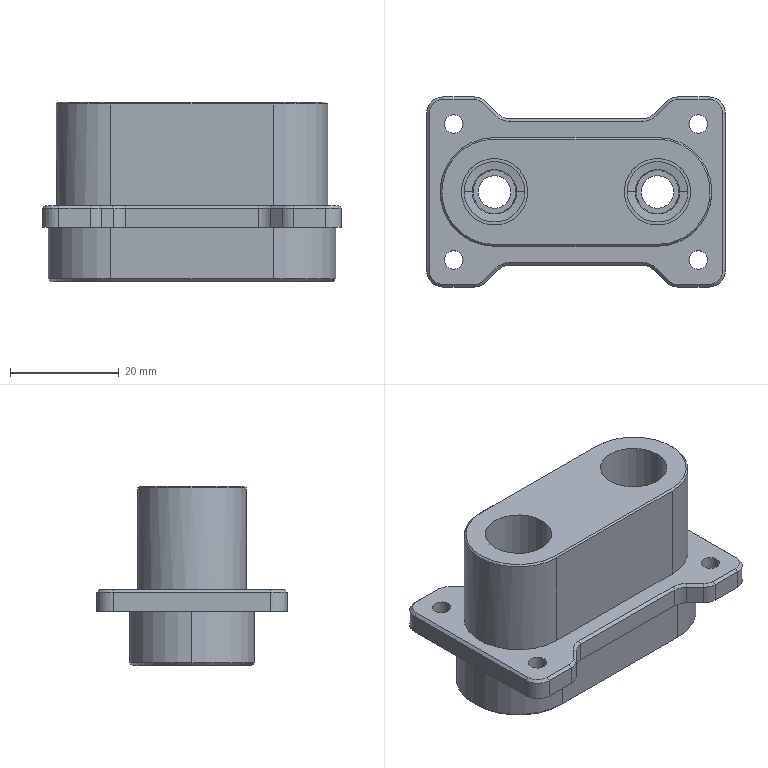NC program | NX | posted with a generic post | part box 55 x 35 x 33 mm
Lines 1 to 866 of 2805:
N10 G17 G21 G94 G90
(ADAPTIVE_MILLING_COPY , TOOL : D6开粗)
N12 T02 M6
N14 G54
N16 G17 G0 G90 X0.026 Y-37.084 S5500 M3
N18 G43 Z30. H2
N20 Z-5.425
N22 G94 G1 X0.007 Y-36.935 Z-6.362 F2500.
N24 X-0.012 Y-36.787 Z-6.733
N26 X-0.03 Y-36.638 Z-7.005
N28 X-0.049 Y-36.489 Z-7.225
N30 X-0.067 Y-36.34 Z-7.409
N32 X-0.086 Y-36.191 Z-7.567
N34 X-0.104 Y-36.042 Z-7.705
N36 X-0.123 Y-35.893 Z-7.825
N38 X-0.142 Y-35.745 Z-7.93
N40 X-0.16 Y-35.596 Z-8.023
N42 X-0.179 Y-35.447 Z-8.104
N44 X-0.197 Y-35.298 Z-8.175
N46 X-0.216 Y-35.149 Z-8.235
N48 X-0.235 Y-35. Z-8.287
N50 X-0.253 Y-34.852 Z-8.33
N52 X-0.272 Y-34.703 Z-8.364
N54 X-0.29 Y-34.554 Z-8.391
N56 X-0.309 Y-34.405 Z-8.41
N58 X-0.327 Y-34.256 Z-8.421
N60 X-0.346 Y-34.107 Z-8.425
N62 X-0.48 Y-33.037
N64 G3 X-0.749 Y-32.605 R0.61
N66 X-2.248 Y-32.071 R3.551
N68 X-6.649 Y-31.766 R30.205
N70 X-18.308 Y-31.715 R976.38
N72 G2 X-20.595 Y-30.24 R3.4
N74 X-21.845 Y-26.899 R7.746
N76 X-22.181 Y-21.414 R38.744
N78 G1 X-22.207 Y-14.414
N80 X-22.226 Y27.67
N82 G2 X-20.867 Y30.02 R3.258
N84 X-17.545 Y31.348 R7.39
N86 X-12.162 Y31.705 R35.743
N88 G1 X-5.862 Y31.731
N90 X18.151 Y31.727
N92 G2 X20.38 Y30.497 R3.21
N94 X21.77 Y27.3 R6.965
N96 X22.165 Y22.422 R29.53
N98 X22.207 Y14.422 R630.04
N100 G1 X22.226 Y-27.666
N102 G2 X20.892 Y-30.028 R3.229
N104 X17.679 Y-31.33 R7.22
N106 X12.598 Y-31.697 R32.844
N108 X1.292 Y-31.713 R705.499
N110 X-2.451 Y-31.255 R126.652
N112 G3 X-10.022 Y-30.942 R80.127
N114 G1 X-16.308 Y-30.914
N116 G2 X-19.675 Y-28.792 R4.529
N118 X-21.021 Y-24.953 R9.492
N120 X-21.382 Y-18.969 R44.715
N122 G1 X-21.408 Y-12.369
N124 X-21.426 Y25.608
N126 G2 X-19.407 Y29.122 R4.47
N128 X-15.588 Y30.527 R9.175
N130 X-9.805 Y30.903 R41.317
N132 G1 X-2.606 Y30.931
N134 X16.068 Y30.929
N136 G2 X19.652 Y28.826 R4.501
N138 X21.015 Y24.99 R9.4
N140 X21.372 Y19.606 R40.78
N142 G1 X21.408 Y12.806
N144 X21.425 Y-25.666
N146 G2 X19.372 Y-29.159 R4.446
N148 X15.63 Y-30.522 R9.178
N150 X9.648 Y-30.903 R42.158
N152 X2.049 Y-30.885 R158.623
N154 X-3.371 Y-30.389 R670.952
N156 G3 X-14.109 Y-30.129 R157.144
N158 G2 X-18.911 Y-27.387 R5.298
N160 X-20.247 Y-23.119 R11.282
N162 X-20.581 Y-17.132 R50.993
N164 G1 X-20.609 Y-10.533
N166 X-20.625 Y23.808
N168 G2 X-18.001 Y28.369 R5.258
N170 X-13.853 Y29.741 R10.794
N172 X-7.668 Y30.105 R48.364
N174 G1 X-0.568 Y30.131
N176 X14.232 Y30.13
N178 G2 X18.871 Y27.455 R5.286
N180 X20.208 Y23.389 R10.832
N182 X20.58 Y17.205 R48.081
N184 G1 X20.609 Y10.105
N186 X20.626 Y-23.766
N188 G2 X17.96 Y-28.403 R5.259
N190 X13.898 Y-29.734 R10.822
N192 X7.813 Y-30.101 R47.178
N194 X-1.396 Y-29.755 R68.035
N196 G3 X-12.922 Y-29.331 R141.705
N198 G2 X-17.987 Y-26.385 R5.801
N200 X-19.397 Y-22.036 R11.657
N202 X-19.785 Y-15.252 R53.401
N204 G1 X-19.809 Y-9.352
N206 X-19.824 Y22.208
N208 G2 X-16.675 Y27.637 R5.869
N210 X-12.391 Y28.944 R12.143
N212 X-5.905 Y29.306 R53.404
N214 G1 X0.195 Y29.33
N216 X12.595 Y29.329
N218 G2 X16.517 Y28.093 R5.985
N220 X18.84 Y24.486 R7.55
N222 X19.639 Y19.664 R19.911
N224 X19.808 Y10.767 R153.746
N226 G1 X19.825 Y-22.033
N228 G2 X18.939 Y-25.568 R6.217
N230 X15.498 Y-28.189 R6.894
N232 X10.805 Y-29.118 R17.241
N234 X-1.373 Y-28.951 R74.067
N236 G3 X-11.736 Y-28.537 R164.985
N238 G2 X-17.272 Y-25.117 R6.289
N240 X-18.625 Y-20.537 R13.086
N242 X-18.985 Y-13.751 R58.838
N244 G1 X-19.01 Y-7.151
N246 X-19.023 Y20.708
N248 G2 X-18.377 Y24.014 R7.257
N250 X-14.856 Y27.168 R6.863
N252 X-10.099 Y28.259 R15.913
N254 X-2.606 Y28.521 R85.519
N256 G1 X2.794 Y28.53
N258 G2 X11.993 Y28.502 R395.137
N260 X17.24 Y25.164 R6.209
N262 X18.615 Y20.593 R12.876
N264 X18.987 Y13.607 R58.872
N266 G1 X19.01 Y6.707
N268 X19.023 Y-20.666
N270 G2 X18.401 Y-23.977 R7.438
N272 X15.007 Y-27.103 R6.724
N274 X10.359 Y-28.231 R15.202
N276 X0.272 Y-28.257 R58.031
N278 G3 X-10.552 Y-27.755 R201.885
N280 G2 X-15.008 Y-26.001 R6.697
N282 X-17.305 Y-21.936 R8.838
N284 X-18.075 Y-16.401 R25.218
N286 X-18.21 Y-5.802 R241.83
N288 G1 X-18.222 Y19.308
N290 G2 X-17.702 Y22.645 R8.715
N292 X-14.186 Y26.175 R6.839
N294 X-9.66 Y27.369 R14.664
N296 X-3.418 Y27.699 R60.201
N298 G1 X-1.732 Y28.037
N300 X-0.018 Y28.151
N302 G2 X3.048 Y27.886 R45.886
N304 G3 X10.276 Y27.724 R125.079
N306 G2 X14.088 Y26.706 R7.126
N308 X16.933 Y23.03 R7.489
N310 X17.97 Y17.953 R18.277
N312 X18.206 Y8.958 R119.092
N314 G1 X18.211 Y5.658
N316 X18.223 Y-19.266
N318 G2 X17.759 Y-22.514 R8.986
N320 X14.288 Y-26.124 R6.789
N322 X9.57 Y-27.378 R14.586
N324 X3.622 Y-27.61 R44.907
N326 G1 X2.938 Y-27.816
N328 X1.192 Y-28.095
N330 X-0.574 Y-28.136
N332 X-2.332 Y-27.94
N334 G3 X-8.02 Y-27.078 R22.47
N336 G2 X-11.094 Y-26.766 R16.798
N338 X-15.546 Y-23.261 R6.842
N340 X-16.967 Y-18.599 R13.627
N342 X-17.379 Y-11.516 R57.069
N344 G1 X-17.41 Y-4.916
N346 X-17.421 Y18.008
N348 G2 X-16.987 Y21.364 R10.177
N350 X-13.465 Y25.214 R6.933
N352 X-8.57 Y26.56 R14.676
N354 X-5.781 Y26.801 R93.594
N356 G3 X-5.044 Y27.145 R25.963
N358 G1 X-3.32 Y27.719
N360 X-1.732 Y28.037
N362 X-0.018 Y28.151
N364 X1.7 Y28.041
N366 X3.389 Y27.707
N368 G3 X6.821 Y27.072 R11.31
N370 G2 X10.345 Y26.863 R61.829
N372 X15.603 Y23.138 R6.806
N374 X16.998 Y18.361 R14.035
N376 X17.379 Y11.575 R58.924
N378 G1 X17.41 Y5.076
N380 X17.422 Y-17.966
N382 G2 X17.003 Y-21.324 R10.338
N384 X13.461 Y-25.219 R6.886
N386 X8.565 Y-26.554 R14.533
N388 X5.873 Y-26.756 R54.643
N390 G1 X4.631 Y-27.306
N392 X3.578 Y-27.624
N394 G3 X3.395 Y-28.682 R0.6
N396 X3.817 Y-28.805 Z-8.387 R0.718
N398 G1 X4.54 Y-28.859 Z-8.325
N400 X5.789 Y-28.949 F15000.
N402 X7.872 Y-28.61
N404 X9.952 Y-28.253
N406 G3 X13.463 Y-27.18 R18.605
N408 X16.658 Y-25.123 R11.437
N410 X18.161 Y-23.033 R7.129
N412 X19.079 Y-19.537 R9.199
N414 X19.299 Y-13.98 R96.733
N416 G1 Y-12.955
N418 X19.1 Y15.604
N420 G3 X18.67 Y19.592 R20.261
N422 X17.517 Y23.435 R19.908
N424 X15.944 Y25.871 R8.654
N426 X13.644 Y27.646 R9.995
N428 X12.259 Y28.284 R6.276
N430 X10.549 Y28.641 R14.684
N432 G1 X5.917 Y29.347
N434 G3 X5.583 Y29.302 R0.62
N436 G1 X4.592 Y28.862
N438 X3.924 Y28.558 Z-8.388 F2500.
N440 G3 X3.668 Y28.215 Z-8.425 R0.618
N442 X4.052 Y27.483 R0.6
N444 G2 X5.616 Y26.875 R8.992
N446 G3 X8.066 Y26.356 R11.217
N448 G2 X11.358 Y25.565 R10.928
N450 X14.97 Y21.835 R7.488
N452 X16.231 Y17.013 R15.728
N454 X16.583 Y10.125 R65.696
N456 G1 X16.611 Y3.525
N458 X16.621 Y-16.766
N460 G2 X16.255 Y-20.134 R11.755
N462 X12.867 Y-24.201 R6.927
N464 X7.916 Y-25.682 R13.585
N466 G3 X7.519 Y-25.769 R5.015
N468 G1 X6.24 Y-26.574
N470 X5.785 Y-26.781
N472 G3 X6.044 Y-27.927 R0.6
N474 G1 X6.402 Y-27.867 Z-8.394
N476 X6.756 Y-27.79 Z-8.363
N478 X7.193 Y-27.699 Z-8.325
N480 X8.48 Y-27.436 F15000.
N482 X9.77 Y-27.189
N484 G3 X13.214 Y-26.033 R13.177
N486 X15.016 Y-24.816 R9.478
N488 G1 X16.078 Y-23.895
N490 G3 X18.001 Y-20.414 R6.496
N492 X18.359 Y-17.157 R16.171
N494 G1 X18.526 Y10.673
N496 G3 X18.139 Y16.503 R40.445
N498 G1 X17.818 Y18.749
N500 G3 X16.226 Y23.279 R14.498
N502 X14.558 Y25.479 R9.819
N504 G1 X14.289 Y25.725
N506 X14.014 Y25.963
N508 X13.477 Y26.404
N510 X12.932 Y26.834
N512 G3 X11.363 Y27.582 R5.165
N514 G1 X10.94 Y27.694
N516 X10.512 Y27.783
N518 X9.093 Y28.028
N520 X7.672 Y28.261
N522 X6.368 Y28.138
N524 X5.974 Y28.102 Z-8.359 F2500.
N526 X5.582 Y28.053 Z-8.393
N528 G3 X5.267 Y27.85 Z-8.425 R0.626
N530 X5.469 Y26.934 R0.6
N532 X7.654 Y25.938 R16.781
N534 G2 X10.526 Y24.882 R17.617
N536 X14.351 Y20.504 R8.316
N538 X15.511 Y15.25 R18.629
N540 X15.801 Y7.058 R96.463
N542 G1 X15.812 Y1.558
N544 X15.82 Y-15.566
N546 G2 X15.454 Y-19.135 R12.951
N548 X11.729 Y-23.494 R7.176
N550 X9.205 Y-24.447 R13.195
N552 G1 X9.077 Y-24.512
N554 X7.736 Y-25.632
N556 X7.482 Y-25.792
N558 G3 X7.526 Y-26.833 R0.6
N560 X8.019 Y-26.87 Z-8.382 R0.693
N562 G1 X8.674 Y-26.751 Z-8.325
N564 X9.854 Y-26.535 F15000.
N566 X10.029 Y-26.475
N568 X11.32 Y-25.788
N570 X12.597 Y-25.074
N572 X13.363 Y-24.616
N574 X14.113 Y-24.134
N576 G3 X15.872 Y-22.292 R6.638
N578 G1 X16.227 Y-21.738
N580 X16.558 Y-21.169
N582 G3 X17.269 Y-18.961 R7.835
N584 X17.56 Y-16.424 R17.3
N586 G1 X17.679 Y-13.314
N588 X17.77 Y-10.203
N590 G3 X17.777 Y-4.347 R163.484
N592 G1 X17.475 Y13.227
N594 G3 X17.014 Y17.579 R24.877
N596 G1 X16.711 Y19.086
N598 G3 X15.597 Y22.089 R11.943
N600 X14.032 Y24.358 R13.938
N602 X12.636 Y25.754 R17.52
N604 X10.213 Y27.228 R6.969
N606 G1 X8.848 Y27.713
N608 X8.706 Y27.744
N610 X8.561 Y27.742
N612 X7.451 Y27.581
N614 X6.726 Y27.469 Z-8.388 F2500.
N616 G3 X6.387 Y27.208 Z-8.425 R0.618
N618 X6.565 Y26.395 R0.6
N620 X9.733 Y24.4 R55.25
N622 G2 X13.805 Y18.977 R9.902
N624 X14.8 Y13.177 R23.848
N626 X15.009 Y3.581 R153.858
N628 G1 X15.012 Y0.281
N630 X15.019 Y-14.419
N632 G2 X14.696 Y-17.995 R14.519
N634 X10.968 Y-22.595 R7.251
N636 G3 X10.285 Y-23.193 R1.337
N638 G1 X9.016 Y-24.563
N640 G3 X9.396 Y-25.623 R0.6
N642 X9.768 Y-25.51 Z-8.391 R0.761
N644 G1 X10.464 Y-25.162 Z-8.325
N646 X11.652 Y-24.563 F15000.
N648 X12.864 Y-23.745
N650 G3 X14.75 Y-21.832 R8.995
N652 X15.929 Y-19.903 R12.896
N654 X16.539 Y-17.664 R7.061
N656 X16.796 Y-14.018 R39.154
N658 G1 X17.044 Y-1.572
N660 G3 X16.767 Y10.131 R134.463
N662 G1 X16.614 Y12.444
N664 X16.448 Y14.756
N666 G3 X15.632 Y19.058 R23.92
N668 X13.13 Y23.811 R13.649
N670 X11.561 Y25.335 R9.763
N672 G1 X10.544 Y26.122
N674 G3 X10.258 Y26.242 R0.638
N676 G1 X9.147 Y26.394
N678 X8.762 Y26.449 Z-8.358 F2500.
N680 X8.376 Y26.491 Z-8.391
N682 G3 X8.014 Y26.356 Z-8.425 R0.625
N684 X7.997 Y25.44 R0.6
N686 G1 X9.292 Y24.306
N688 G2 X11.706 Y21.209 R20.425
N690 X13.654 Y15.447 R15.948
N692 X14.164 Y7.971 R54.842
N694 X14.213 Y-1.029 R663.025
N696 G1 X14.218 Y-13.229
N698 G2 X13.949 Y-16.812 R17.084
N700 X11.958 Y-20.43 R7.248
N702 X10.437 Y-22.973 R12.961
N704 G3 X11.335 Y-23.758 R0.6
N706 G1 X12.21 Y-22.979 Z-8.325
N708 X12.984 Y-22.291 F15000.
N710 X13.667 Y-21.597
N712 G3 X14.332 Y-20.593 R4.261
N714 G1 X14.979 Y-19.202
N716 G3 X15.873 Y-15.387 R11.666
N718 X16.024 Y-11.001 R56.254
N720 G1 X15.892 Y9.138
N722 G3 X15.431 Y15.405 R48.944
N724 X14.261 Y19.92 R21.282
N726 G1 X13.065 Y23.012
N728 G3 X12.703 Y23.362 R0.604
N730 G1 X11.749 Y23.694
N732 X11.39 Y23.823 Z-8.358 F2500.
N734 X11.026 Y23.937 Z-8.39
N736 G3 X10.631 Y23.867 Z-8.425 R0.623
N738 X10.428 Y23.012 R0.6
N740 G1 X11.386 Y21.581
N742 X12.148 Y20.037
N744 X12.701 Y18.407
N746 X13.037 Y16.718
N748 G2 X13.164 Y13.611 R36.952
N750 X13.412 Y-1.277 R306.962
N752 X13.389 Y-13.776 R717.094
N754 X13.07 Y-16.19 R11.959
N756 G1 X13.031 Y-16.764
N758 X12.676 Y-18.496
N760 X12.093 Y-20.164
N762 X11.957 Y-20.432
N764 G3 X12.396 Y-21.296 R0.6
N766 X12.937 Y-21.122 Z-8.375 R0.686
N768 G1 X13.411 Y-20.78 Z-8.325
N770 X14.258 Y-20.17 F15000.
N772 G3 X14.503 Y-19.749 R0.604
N774 G1 X14.909 Y-16.007
N776 G3 X15.137 Y-10.999 R52.234
N778 G1 X15.081 Y8.19
N780 X15.058 Y10.163
N782 X15.014 Y12.137
N784 X15.002 Y12.23
N786 X14.98 Y12.322
N788 X14.621 Y13.338
N790 X14.455 Y13.81 Z-8.368 F2500.
N792 X14.281 Y14.279 Z-8.41
N794 X14.181 Y14.418 Z-8.425
N796 G3 X13.15 Y14.001 R0.6
N798 G1 Y-14.999
N800 X13.069 Y-16.197
N802 G3 X13.351 Y-16.746 R0.601
N804 G1 X13.784 Y-16.937 Z-8.385
N806 X14.223 Y-17.112 Z-8.344
N808 X14.432 Y-17.197 Z-8.325
N810 X14.608 Y-17.269 F15000.
N812 X14.771 Y-17.368
N814 G2 X14.933 Y-18.061 R0.601
N816 G1 X14.287 Y-19.574
N818 X13.614 Y-21.075
N820 G2 X12.42 Y-23.382 R33.829
N822 X10.125 Y-26.125 R11.41
N824 X6.911 Y-28.293 R13.574
N826 X1.886 Y-29.856 R16.229
N828 X-0.608 Y-29.935 R12.825
N830 G1 X-2.729 Y-29.794
N832 G2 X-3.265 Y-29.364 R0.601
N834 G1 X-3.305 Y-29.224
N836 X-3.635 Y-28.1 Z-8.425 F2500.
N838 X-3.689 Y-27.913
N840 X-3.77 Y-27.735
N842 G3 X-4.047 Y-27.511 R0.616
N844 X-6.347 Y-26.687 R15.113
N846 X-9.396 Y-26.206 R84.88
N848 G2 X-14.986 Y-21.824 R7.426
N850 X-16.258 Y-16.806 R16.186
N852 X-16.592 Y-9.316 R75.342
N854 G1 X-16.611 Y-3.116
N856 X-16.621 Y16.708
N858 G2 X-16.24 Y20.174 R11.827
N860 X-12.497 Y24.399 R7.085
N862 X-7.698 Y25.73 R14.824
N864 G1 X-7.45 Y25.805
N866 G2 X-5.599 Y26.871 R9.59
N868 G3 X-5.922 Y28.006 R0.6
N870 G1 X-7.07 Y27.774 Z-8.325
N872 X-8.326 Y27.52 F15000.
N874 X-9.584 Y27.279
N876 G3 X-13.685 Y25.8 R13.984
N878 X-15.901 Y24.182 R13.533
N880 X-17.03 Y22.766 R5.282
N882 G1 X-17.369 Y22.138
N884 X-17.7 Y21.505
N886 G3 X-18.398 Y18.423 R7.16
N888 G1 Y-12.358
N890 G3 X-17.976 Y-17.45 R31.028
N892 G1 X-17.807 Y-18.472
N894 X-17.609 Y-19.489
N896 G3 X-16.771 Y-22.137 R15.239
N898 X-15.761 Y-23.947 R10.845
N900 G1 X-14.924 Y-25.146
N902 G3 X-14.315 Y-25.821 R3.853
N904 X-12.965 Y-26.756 R16.993
N906 X-11.657 Y-27.393 R8.899
N908 G1 X-10.915 Y-27.682
N910 X-10.169 Y-27.96
N912 G3 X-8.713 Y-28.21 R5.251
N914 G1 X-7.752 Y-28.233
N916 X-6.434 Y-28.13
N918 X-6.027 Y-28.099 Z-8.36 F2500.
N920 X-5.62 Y-28.059 Z-8.395
N922 G3 X-5.318 Y-27.885 Z-8.425 R0.63
N924 X-5.533 Y-26.917 R0.6
N926 G2 X-6.714 Y-26.295 R25.203
N928 G3 X-9.123 Y-25.497 R31.002
N930 G2 X-14.334 Y-20.577 R8.267
N932 X-15.506 Y-15.326 R18.584
N934 X-15.799 Y-7.234 R94.021
N936 G1 X-15.812 Y-1.734
N938 X-15.82 Y15.508
N940 G2 X-15.466 Y19.079 R13.231
N942 X-11.838 Y23.433 R7.139
N944 X-9.14 Y24.478 R13.37
N946 G1 X-9.02 Y24.543
N948 G2 X-7.431 Y25.817 R10.355
N950 G3 X-7.486 Y26.847 R0.6
N952 X-7.98 Y26.887 Z-8.382 R0.692
N954 G1 X-8.634 Y26.77 Z-8.325
N956 X-9.802 Y26.56 F15000.
N958 X-9.891 Y26.534
N960 X-9.978 Y26.499
N962 X-11.269 Y25.813
N964 X-12.546 Y25.099
N966 X-13.469 Y24.543
N968 X-14.373 Y23.96
N970 G3 X-16.402 Y21.488 R6.136
N972 X-17.352 Y18.37 R10.617
N974 X-17.6 Y15.46 R29.323
N976 G1 X-17.722 Y11.922
N978 X-17.811 Y8.384
N980 G3 X-17.788 Y1.552 R184.951
N982 G1 X-17.438 Y-14.19
N984 G3 X-16.937 Y-18.169 R19.687
N986 X-15.776 Y-21.734 R17.491
N988 X-14.101 Y-24.424 R13.55
N990 X-11.224 Y-26.603 R8.113
N992 G1 X-8.844 Y-27.685
N994 G3 X-8.511 Y-27.733 R0.62
N996 G1 X-7.422 Y-27.577
N998 X-7.044 Y-27.527 Z-8.358 F2500.
N1000 X-6.67 Y-27.461 Z-8.39
N1002 G3 X-6.35 Y-27.216 Z-8.425 R0.623
N1004 X-6.561 Y-26.367 R0.6
N1006 G2 X-7.807 Y-25.558 R8.109
N1008 X-10.398 Y-23.949 R30.78
N1010 X-13.846 Y-18.876 R9.948
N1012 X-14.81 Y-13.07 R24.557
N1014 X-15.009 Y-3.573 R159.843
N1016 G1 X-15.019 Y13.827
N1018 G2 X-14.783 Y17.613 R19.265
N1020 X-11.048 Y22.552 R7.255
N1022 G3 X-10.437 Y23.001 R1.45
N1024 G1 X-9.304 Y24.294
N1026 X-9.004 Y24.558
N1028 G3 X-9.459 Y25.606 R0.6
N1030 G1 X-9.645 Y25.555 Z-8.409
N1032 X-9.818 Y25.471 Z-8.392
N1034 X-10.521 Y25.12 Z-8.325
N1036 X-11.64 Y24.558 F15000.
N1038 X-12.852 Y23.74
N1040 G3 X-14.738 Y21.827 R8.995
N1042 X-15.948 Y19.754 R10.099
N1044 X-16.644 Y16.572 R9.71
N1046 X-16.857 Y11.086 R153.327
N1048 G1 X-17.061 Y0.471
N1050 G3 X-16.775 Y-10.499 R121.225
N1052 G1 X-16.636 Y-12.455
N1054 X-16.488 Y-14.41
N1056 G3 X-15.885 Y-18.117 R28.072
N1058 G1 X-15.547 Y-19.541
N1060 G3 X-13.744 Y-23.094 R10.045
N1062 X-11.441 Y-25.413 R11.629
N1064 G1 X-10.231 Y-26.321
N1066 X-10.102 Y-26.393
N1068 X-9.961 Y-26.435
N1070 X-8.86 Y-26.604
N1072 X-8.044 Y-26.722 Z-8.395 F2500.
N1074 G3 X-7.715 Y-26.627 Z-8.425 R0.631
N1076 X-7.684 Y-25.639 R0.6
N1078 G1 X-8.441 Y-25.082
N1080 X-9.631 Y-23.952
N1082 G2 X-11.76 Y-21.116 R22.541
N1084 X-13.687 Y-15.26 R16.031
N1086 X-14.165 Y-7.981 R56.737
N1088 X-14.212 Y1.019 R665.381
N1090 G1 X-14.217 Y13.119
N1092 G2 X-13.926 Y16.899 R16.988
N1094 X-11.945 Y20.447 R7.372
N1096 G1 X-11.391 Y21.572
N1098 X-10.447 Y22.986
N1100 G3 X-11.294 Y23.807 R0.6
N1102 G1 X-12.173 Y23.033 Z-8.325
N1104 X-12.994 Y22.303 F15000.
N1106 X-13.677 Y21.61
N1108 G3 X-14.342 Y20.605 R4.261
N1110 G1 X-14.989 Y19.214
N1112 G3 X-15.863 Y15.398 R11.713
N1114 X-16.009 Y11.011 R59.384
N1116 G1 X-15.903 Y-8.031
N1118 G3 X-15.556 Y-14.261 R67.701
N1120 X-14.949 Y-18.038 R26.203
N1122 X-14.376 Y-19.861 R17.077
N1124 G1 X-13.307 Y-22.683
N1126 G3 X-12.939 Y-23.039 R0.603
N1128 G1 X-11.99 Y-23.361
N1130 X-11.633 Y-23.485 Z-8.357 F2500.
N1132 X-11.271 Y-23.596 Z-8.39
N1134 G3 X-10.872 Y-23.518 Z-8.425 R0.623
N1136 X-10.671 Y-22.683 R0.6
N1138 G1 X-11.545 Y-21.295
N1140 X-12.239 Y-19.808
N1142 X-12.742 Y-18.247
N1144 G2 X-13.15 Y-14.998 R15.398
N1146 G3 X-13.31 Y-9.779 R147.475
N1148 G2 X-13.414 Y3.62 R551.636
N1150 X-13.385 Y13.82 R469.393
N1152 X-13.073 Y16.169 R11.91
N1154 G1 X-13.038 Y16.717
N1156 X-12.702 Y18.403
N1158 X-12.15 Y20.03
N1160 X-11.929 Y20.479
N1162 G3 X-12.37 Y21.336 R0.6
N1164 X-12.913 Y21.163 Z-8.375 R0.685
N1166 G1 X-13.386 Y20.822 Z-8.325
N1168 X-14.23 Y20.215 F15000.
N1170 G3 X-14.476 Y19.796 R0.604
N1172 G1 X-14.9 Y16.056
N1174 G3 X-15.138 Y11.048 R50.052
N1176 G1 X-15.084 Y-8.067
N1178 X-15.06 Y-10.151
N1180 X-15.014 Y-12.234
N1182 X-15.002 Y-12.328
N1184 X-14.98 Y-12.42
N1186 X-14.621 Y-13.436
N1188 X-14.455 Y-13.908 Z-8.368 F2500.
N1190 X-14.281 Y-14.377 Z-8.41
N1192 X-14.181 Y-14.515 Z-8.425
N1194 G3 X-13.15 Y-14.098 R0.6
N1196 G1 Y15.002
N1198 X-13.071 Y16.199
N1200 G3 X-13.484 Y16.814 R0.607
N1202 G1 X-14.448 Y17.135
N1204 X-14.59 Y17.183 Z-8.421
N1206 X-14.732 Y17.231 Z-8.41
N1208 X-14.874 Y17.278 Z-8.391
N1210 X-15.017 Y17.326 Z-8.364
N1212 X-15.159 Y17.373 Z-8.33
N1214 X-15.301 Y17.421 Z-8.287
N1216 X-15.444 Y17.468 Z-8.235
N1218 X-15.586 Y17.516 Z-8.175
N1220 X-15.728 Y17.563 Z-8.104
N1222 X-15.87 Y17.611 Z-8.023
N1224 X-16.013 Y17.658 Z-7.93
N1226 X-16.155 Y17.706 Z-7.825
N1228 X-16.297 Y17.753 Z-7.705
N1230 X-16.439 Y17.801 Z-7.567
N1232 X-16.582 Y17.848 Z-7.409
N1234 X-16.724 Y17.896 Z-7.225
N1236 X-16.866 Y17.944 Z-7.005
N1238 X-17.008 Y17.991 Z-6.733
N1240 X-17.151 Y18.039 Z-6.362
N1242 X-17.293 Y18.086 Z-5.425
N1244 G0 Z30.
N1246 X2.166 Y-32.232
N1248 Z3.105
N1250 G1 X2.097 Y-32.099 Z2.168
N1252 X2.027 Y-31.966 Z1.797
N1254 X1.957 Y-31.833 Z1.524
N1256 X1.888 Y-31.7 Z1.305
N1258 X1.818 Y-31.567 Z1.12
N1260 X1.749 Y-31.434 Z0.962
N1262 X1.679 Y-31.301 Z0.825
N1264 X1.61 Y-31.168 Z0.705
N1266 X1.54 Y-31.035 Z0.599
N1268 X1.471 Y-30.903 Z0.506
N1270 X1.401 Y-30.77 Z0.425
N1272 X1.331 Y-30.637 Z0.355
N1274 X1.262 Y-30.504 Z0.294
N1276 X1.192 Y-30.371 Z0.243
N1278 X1.123 Y-30.238 Z0.2
N1280 X1.053 Y-30.105 Z0.165
N1282 X0.984 Y-29.972 Z0.138
N1284 X0.914 Y-29.839 Z0.12
N1286 X0.845 Y-29.706 Z0.108
N1288 X0.775 Y-29.574 Z0.105
N1290 G3 X0.1 Y-28.323 R42.578
N1292 X-0.963 Y-27.743 R2.759
N1294 G1 X-1.656 Y-27.699
N1296 X-3.301 Y-27.374
N1298 X-4.889 Y-26.836
N1300 X-6.394 Y-26.096
N1302 X-7.789 Y-25.166
N1304 X-9.05 Y-24.061
N1306 X-10.157 Y-22.801
N1308 X-11.089 Y-21.407
N1310 X-11.831 Y-19.903
N1312 X-12.371 Y-18.316
N1314 X-12.698 Y-16.671
N1316 X-12.808 Y-14.998
N1318 Y15.002
N1320 G2 X-12.419 Y18.131 R14.92
N1322 X-11.278 Y21.07 R14.917
N1324 X-9.454 Y23.642 R14.917
N1326 X-7.056 Y25.69 R14.917
N1328 G1 X-5.687 Y26.477
N1330 X-4.086 Y27.14
N1332 X-2.41 Y27.58
N1334 X-0.69 Y27.79
N1336 X1.043 Y27.766
N1338 X2.756 Y27.509
N1340 X4.419 Y27.022
N1342 X6.002 Y26.316
N1344 X7.474 Y25.402
N1346 X8.809 Y24.298
N1348 X9.984 Y23.024
N1350 X10.975 Y21.603
N1352 X11.766 Y20.061
N1354 X12.341 Y18.426
N1356 X12.69 Y16.729
N1358 X12.808 Y15.001
N1360 Y-14.999
N1362 X12.698 Y-16.67
N1364 X12.372 Y-18.312
N1366 X11.834 Y-19.897
N1368 X11.094 Y-21.398
N1370 X10.165 Y-22.79
N1372 X9.062 Y-24.049
N1374 X7.805 Y-25.154
N1376 X6.414 Y-26.085
N1378 X4.913 Y-26.826
N1380 X3.329 Y-27.366
N1382 X1.688 Y-27.695
N1384 X0.019 Y-27.806
N1386 X-0.979 Y-27.742
N1388 G3 X-1.622 Y-28.399 R0.606
N1390 G1 X-1.556 Y-29.173
N1392 X-1.543 Y-29.322 Z0.108
N1394 X-1.53 Y-29.472 Z0.12
N1396 X-1.517 Y-29.621 Z0.138
N1398 X-1.504 Y-29.771 Z0.165
N1400 X-1.492 Y-29.92 Z0.2
N1402 X-1.479 Y-30.07 Z0.243
N1404 X-1.466 Y-30.219 Z0.294
N1406 X-1.453 Y-30.369 Z0.355
N1408 X-1.44 Y-30.518 Z0.425
N1410 X-1.428 Y-30.667 Z0.506
N1412 X-1.415 Y-30.817 Z0.599
N1414 X-1.402 Y-30.966 Z0.705
N1416 X-1.389 Y-31.116 Z0.825
N1418 X-1.376 Y-31.265 Z0.962
N1420 X-1.364 Y-31.415 Z1.12
N1422 X-1.351 Y-31.564 Z1.305
N1424 X-1.338 Y-31.714 Z1.524
N1426 X-1.325 Y-31.863 Z1.797
N1428 X-1.312 Y-32.013 Z2.168
N1430 X-1.3 Y-32.162 Z3.105
N1432 G0 Z30.
N1434 X2.164 Y-31.938
N1436 Z3.15
N1438 G1 X2.094 Y-31.805 Z2.213
N1440 X2.024 Y-31.673 Z1.842
N1442 X1.954 Y-31.54 Z1.57
N1444 X1.884 Y-31.407 Z1.35
N1446 X1.814 Y-31.274 Z1.166
N1448 X1.744 Y-31.142 Z1.008
N1450 X1.674 Y-31.009 Z0.87
N1452 X1.604 Y-30.876 Z0.75
N1454 X1.534 Y-30.744 Z0.645
N1456 X1.464 Y-30.611 Z0.552
N1458 X1.394 Y-30.478 Z0.471
N1460 X1.324 Y-30.346 Z0.4
N1462 X1.254 Y-30.213 Z0.34
N1464 X1.184 Y-30.08 Z0.288
N1466 X1.115 Y-29.947 Z0.245
N1468 X1.045 Y-29.815 Z0.211
N1470 X0.975 Y-29.682 Z0.184
N1472 X0.905 Y-29.549 Z0.165
N1474 X0.835 Y-29.417 Z0.154
N1476 X0.765 Y-29.284 Z0.15
N1478 G3 X0.058 Y-27.98 R63.52
N1480 X-1.235 Y-27.285 R3.73
N1482 G2 X-5.088 Y-25.735 R30.616
N1484 X-11.805 Y-15.606 R12.278
N1486 X-12.004 Y-8.711 R82.573
N1488 G1 X-12.007 Y-5.011
N1490 X-12.006 Y13.289
N1492 G2 X-11.288 Y18.517 R16.608
N1494 X11.332 Y18.223 R11.813
N1496 X11.929 Y13.673 R19.418
N1498 X12.007 Y4.773 R297.549
N1500 G1 X12.006 Y-13.327
N1502 G2 X11.21 Y-18.742 R16.264
N1504 X2.559 Y-26.488 R11.822
N1506 X-1.108 Y-26.218 R9.5
N1508 X-7.611 Y-22.664 R13.347
N1510 X-10.757 Y-16.18 R11.753
N1512 X-11.167 Y-10.5 R40.47
N1514 X-11.207 Y-2.6 R628.679
N1516 G1 X-11.206 Y12.
N1518 G2 X-10.664 Y17.257 R20.516
N1520 X-3.359 Y25.22 R11.223
N1522 X10.572 Y17.09 R10.811
N1524 X11.138 Y11.627 R29.212
N1526 X11.207 Y2.728 R382.263
N1528 G1 X11.206 Y-11.972
N1530 G2 X10.67 Y-17.23 R20.572
N1532 X4.283 Y-24.86 R11.242
N1534 X-0.832 Y-25.204 R8.981
N1536 X-8.252 Y-20.166 R11.189
N1538 X-9.98 Y-14.968 R13.691
N1540 X-10.379 Y-8.285 R52.522
N1542 G1 X-10.407 Y-1.685
N1544 X-10.406 Y10.915
N1546 G2 X-9.983 Y16.088 R24.676
N1548 X-5.905 Y22.723 R11.044
N1550 X9.283 Y17.89 R9.778
N1552 X10.224 Y12.588 R20.833
N1554 X10.406 Y2.991 R154.319
N1556 G1 X10.407 Y-10.209
N1558 G2 X10.099 Y-15.493 R30.622
N1560 X6.86 Y-21.905 R11.503
N1562 X-0.494 Y-24.165 R8.288
N1564 X-8.408 Y-17.336 R9.997
N1566 X-9.409 Y-11.741 R21.982
N1568 X-9.605 Y-2.545 R145.442
N1570 G1 X-9.607 Y9.155
N1572 G2 X-9.325 Y14.642 R35.663
N1574 X-6.808 Y20.436 R11.473
N1576 X5.721 Y21.408 R8.773
N1578 X8.678 Y16.374 R10.28
N1580 X9.476 Y10.54 R27.086
N1582 X9.606 Y-0.158 R248.291
N1584 X9.573 Y-11.858 R673.787
N1586 X8.654 Y-17.258 R17.105
N1588 X5.13 Y-21.909 R9.391
N1590 X-1.877 Y-22.67 R7.975
N1592 X-7.13 Y-17.721 R9.023
N1594 X-8.456 Y-12.407 R17.631
N1596 X-8.795 Y-4.218 R82.05
N1598 X-8.772 Y11.082 R808.863
N1600 X-7.967 Y16.301 R18.121
N1602 X-3.887 Y21.445 R9.131
N1604 X6.508 Y18.695 R7.695
N1606 X8.237 Y13.825 R13.395
N1608 X8.76 Y6.851 R47.094
N1610 X8.773 Y-11.048 R777.873
N1612 X7.976 Y-16.269 R18.202
N1614 X5.11 Y-20.517 R8.792
N1616 X-4.101 Y-20.018 R7.209
N1618 X-6.872 Y-15.435 R10.081
N1620 X-7.827 Y-9.425 R25.525
N1622 X-8.005 Y0.572 R180.737
N1624 X-7.958 Y10.671 R365.288
N1626 X-7.12 Y15.783 R17.35
N1628 X-3.502 Y20.335 R8.312
N1630 X5.067 Y18.676 R6.67
N1632 X7.165 Y14.179 R11.04
N1634 X7.888 Y8.13 R31.927
N1636 X8.006 Y-2.868 R291.66
N1638 X7.939 Y-11.067 R204.278
N1640 X6.977 Y-16.154 R15.933
N1642 X3.832 Y-19.911 R7.205
N1644 X1.733 Y-20.609 R6.262
N1646 G1 X1.151 Y-20.785
N1648 X0. Y-20.899
N1650 X-1.151 Y-20.785
N1652 X-2.258 Y-20.45
N1654 X-3.278 Y-19.904
N1656 X-4.172 Y-19.171
N1658 X-4.906 Y-18.277
N1660 X-5.451 Y-17.257
N1662 G2 X-7.051 Y-8.171 R32.415
N1664 X-7.205 Y1.726 R210.068
N1666 X-7.141 Y10.325 R225.514
N1668 X-6.274 Y15.229 R16.268
N1670 X-5.672 Y16.529 R13.645
N1672 G1 X-5.451 Y17.259
N1674 X-4.906 Y18.279
N1676 X-4.172 Y19.173
N1678 X-3.278 Y19.907
N1680 X-2.258 Y20.452
N1682 X-1.151 Y20.788
N1684 X0. Y20.901
N1686 X1.151 Y20.788
N1688 X2.258 Y20.452
N1690 X3.278 Y19.907
N1692 X4.172 Y19.173
N1694 X4.906 Y18.279
N1696 X5.451 Y17.259
N1698 G2 X7.06 Y7.869 R34.29
N1700 X7.206 Y-3.929 R268.724
N1702 X7.097 Y-11.027 R112.986
N1704 X6.115 Y-15.6 R14.031
N1706 G1 X5.708 Y-16.408
N1708 X5.451 Y-17.257
N1710 X4.906 Y-18.277
N1712 X4.172 Y-19.171
N1714 X3.278 Y-19.904
N1716 X2.258 Y-20.45
N1718 X1.151 Y-20.785
N1720 X0. Y-20.899
N1722 X-1.151 Y-20.785
N1724 X-2.258 Y-20.45
N1726 X-3.278 Y-19.904
N1728 X-4.172 Y-19.171
N1730 X-4.906 Y-18.277